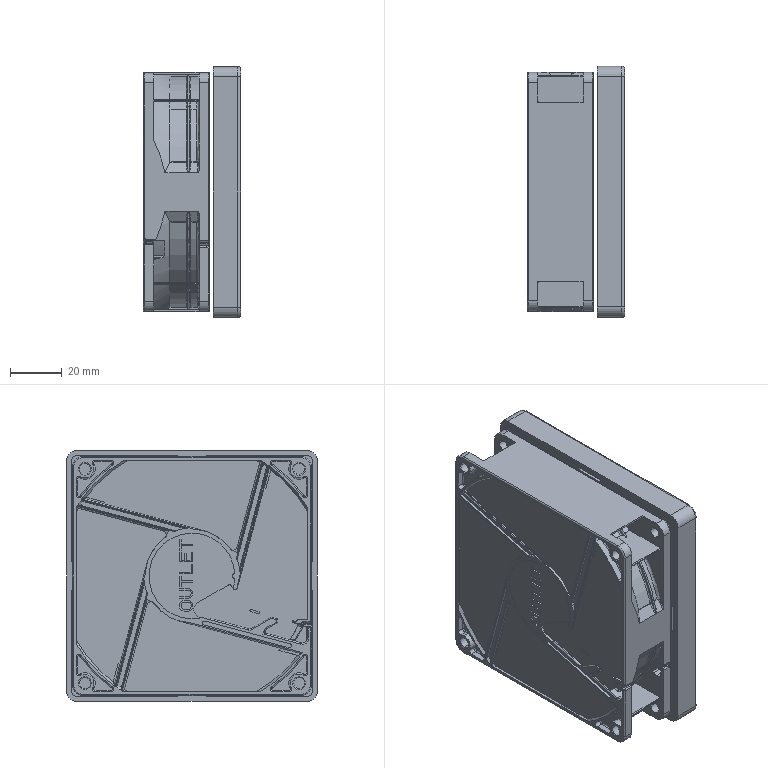Part | SolidWorks | 4 solids | 1414 faces | box 37.408 x 96.6 x 96.6 mm | volume 223267 mm3 | plane 834 | cylinder 335 | torus 164 | cone 36 | spline 32 | sphere 13 | commonest cylinder face diameters 1 x63 2 x48 0.6 x19 90 x19 4.3 x16 8 x16